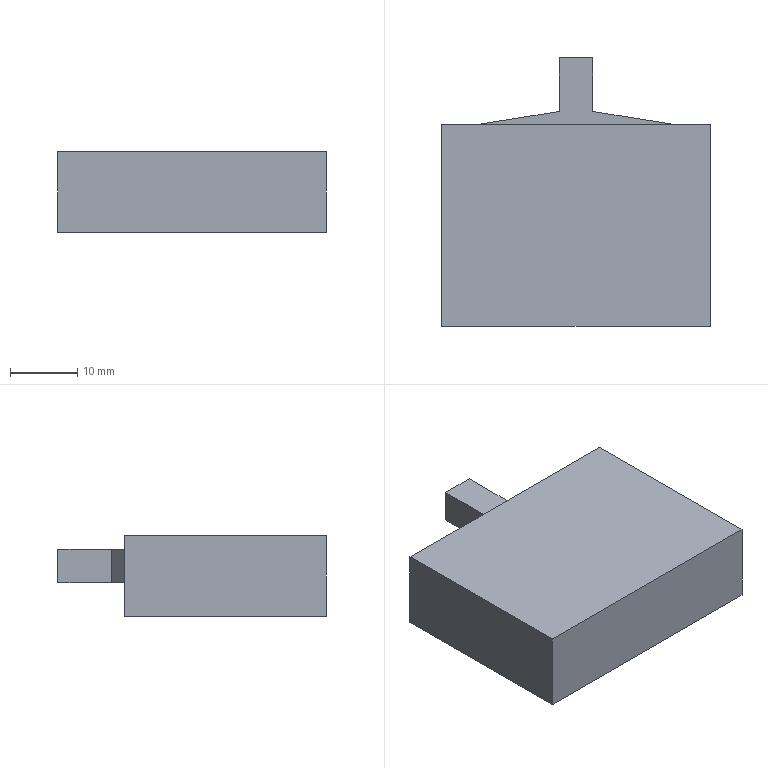Part | SolidWorks | features Extrusion 1, ICE 1 | 1 solid | 13 faces | box 40 x 40 x 12 mm | volume 14775 mm3 | plane 13
STEP:
#1=CARTESIAN_POINT('',(0.,0.,0.));
#2=VERTEX_POINT('',#1);
#3=CARTESIAN_POINT('',(0.,-30.,0.));
#4=VERTEX_POINT('',#3);
#5=CARTESIAN_POINT('',(0.,0.,0.));
#6=DIRECTION('',(0.,-1.,0.));
#7=VECTOR('',#6,1000.);
#8=LINE('',#5,#7);
#9=EDGE_CURVE('',#2,#4,#8,.T.);
#10=ORIENTED_EDGE('',*,*,#9,.T.);
#11=CARTESIAN_POINT('',(0.,-30.,12.));
#12=VERTEX_POINT('',#11);
#13=CARTESIAN_POINT('',(0.,-30.,12.));
#14=DIRECTION('',(0.,0.,-1.));
#15=VECTOR('',#14,1000.);
#16=LINE('',#13,#15);
#17=EDGE_CURVE('',#12,#4,#16,.T.);
#18=ORIENTED_EDGE('',*,*,#17,.F.);
#19=CARTESIAN_POINT('',(0.,0.,12.));
#20=VERTEX_POINT('',#19);
#21=CARTESIAN_POINT('',(0.,0.,12.));
#22=DIRECTION('',(0.,-1.,0.));
#23=VECTOR('',#22,1000.);
#24=LINE('',#21,#23);
#25=EDGE_CURVE('',#20,#12,#24,.T.);
#26=ORIENTED_EDGE('',*,*,#25,.F.);
#27=CARTESIAN_POINT('',(0.,0.,12.));
#28=DIRECTION('',(0.,0.,-1.));
#29=VECTOR('',#28,1000.);
#30=LINE('',#27,#29);
#31=EDGE_CURVE('',#20,#2,#30,.T.);
#32=ORIENTED_EDGE('',*,*,#31,.T.);
#33=EDGE_LOOP('',(#10,#18,#26,#32));
#34=FACE_OUTER_BOUND('',#33,.T.);
#35=CARTESIAN_POINT('',(0.,0.,12.));
#36=DIRECTION('',(1.,0.,0.));
#37=DIRECTION('',(0.,1.,0.));
#38=AXIS2_PLACEMENT_3D('',#35,#36,#37);
#39=PLANE('',#38);
#40=ADVANCED_FACE('',(#34),#39,.F.);
#41=CARTESIAN_POINT('',(40.,-30.,0.));
#42=VERTEX_POINT('',#41);
#43=CARTESIAN_POINT('',(0.,-30.,0.));
#44=DIRECTION('',(1.,0.,0.));
#45=VECTOR('',#44,1000.);
#46=LINE('',#43,#45);
#47=EDGE_CURVE('',#4,#42,#46,.T.);
#48=ORIENTED_EDGE('',*,*,#47,.T.);
#49=CARTESIAN_POINT('',(40.,-30.,12.));
#50=VERTEX_POINT('',#49);
#51=CARTESIAN_POINT('',(40.,-30.,12.));
#52=DIRECTION('',(0.,0.,-1.));
#53=VECTOR('',#52,1000.);
#54=LINE('',#51,#53);
#55=EDGE_CURVE('',#50,#42,#54,.T.);
#56=ORIENTED_EDGE('',*,*,#55,.F.);
#57=CARTESIAN_POINT('',(0.,-30.,12.));
#58=DIRECTION('',(1.,0.,0.));
#59=VECTOR('',#58,1000.);
#60=LINE('',#57,#59);
#61=EDGE_CURVE('',#12,#50,#60,.T.);
#62=ORIENTED_EDGE('',*,*,#61,.F.);
#63=ORIENTED_EDGE('',*,*,#17,.T.);
#64=EDGE_LOOP('',(#48,#56,#62,#63));
#65=FACE_OUTER_BOUND('',#64,.T.);
#66=CARTESIAN_POINT('',(0.,-30.,12.));
#67=DIRECTION('',(0.,1.,0.));
#68=DIRECTION('',(0.,0.,1.));
#69=AXIS2_PLACEMENT_3D('',#66,#67,#68);
#70=PLANE('',#69);
#71=ADVANCED_FACE('',(#65),#70,.F.);
#72=CARTESIAN_POINT('',(40.,0.,0.));
#73=VERTEX_POINT('',#72);
#74=CARTESIAN_POINT('',(40.,0.,0.));
#75=DIRECTION('',(0.,1.,0.));
#76=VECTOR('',#75,1000.);
#77=LINE('',#74,#76);
#78=EDGE_CURVE('',#42,#73,#77,.T.);
#79=ORIENTED_EDGE('',*,*,#78,.T.);
#80=CARTESIAN_POINT('',(40.,0.,12.));
#81=VERTEX_POINT('',#80);
#82=CARTESIAN_POINT('',(40.,0.,12.));
#83=DIRECTION('',(0.,0.,-1.));
#84=VECTOR('',#83,1000.);
#85=LINE('',#82,#84);
#86=EDGE_CURVE('',#81,#73,#85,.T.);
#87=ORIENTED_EDGE('',*,*,#86,.F.);
#88=CARTESIAN_POINT('',(40.,0.,12.));
#89=DIRECTION('',(0.,1.,0.));
#90=VECTOR('',#89,1000.);
#91=LINE('',#88,#90);
#92=EDGE_CURVE('',#50,#81,#91,.T.);
#93=ORIENTED_EDGE('',*,*,#92,.F.);
#94=ORIENTED_EDGE('',*,*,#55,.T.);
#95=EDGE_LOOP('',(#79,#87,#93,#94));
#96=FACE_OUTER_BOUND('',#95,.T.);
#97=CARTESIAN_POINT('',(40.,0.,12.));
#98=DIRECTION('',(-1.,0.,0.));
#99=DIRECTION('',(0.,-1.,0.));
#100=AXIS2_PLACEMENT_3D('',#97,#98,#99);
#101=PLANE('',#100);
#102=ADVANCED_FACE('',(#96),#101,.F.);
#103=CARTESIAN_POINT('',(5.,0.,10.));
#104=VERTEX_POINT('',#103);
#105=CARTESIAN_POINT('',(5.,0.,5.));
#106=VERTEX_POINT('',#105);
#107=CARTESIAN_POINT('',(5.,0.,10.));
#108=DIRECTION('',(0.,0.,-1.));
#109=VECTOR('',#108,1000.);
#110=LINE('',#107,#109);
#111=EDGE_CURVE('',#104,#106,#110,.T.);
#112=ORIENTED_EDGE('',*,*,#111,.T.);
#113=CARTESIAN_POINT('',(35.,0.,5.));
#114=VERTEX_POINT('',#113);
#115=CARTESIAN_POINT('',(0.,0.,5.));
#116=DIRECTION('',(1.,0.,0.));
#117=VECTOR('',#116,1000.);
#118=LINE('',#115,#117);
#119=EDGE_CURVE('',#106,#114,#118,.T.);
#120=ORIENTED_EDGE('',*,*,#119,.T.);
#121=CARTESIAN_POINT('',(35.,0.,10.));
#122=VERTEX_POINT('',#121);
#123=CARTESIAN_POINT('',(35.,0.,10.));
#124=DIRECTION('',(0.,0.,-1.));
#125=VECTOR('',#124,1000.);
#126=LINE('',#123,#125);
#127=EDGE_CURVE('',#122,#114,#126,.T.);
#128=ORIENTED_EDGE('',*,*,#127,.F.);
#129=CARTESIAN_POINT('',(0.,0.,10.));
#130=DIRECTION('',(1.,0.,0.));
#131=VECTOR('',#130,1000.);
#132=LINE('',#129,#131);
#133=EDGE_CURVE('',#104,#122,#132,.T.);
#134=ORIENTED_EDGE('',*,*,#133,.F.);
#135=EDGE_LOOP('',(#112,#120,#128,#134));
#136=FACE_BOUND('',#135,.T.);
#137=CARTESIAN_POINT('',(0.,0.,0.));
#138=DIRECTION('',(-1.,0.,0.));
#139=VECTOR('',#138,1000.);
#140=LINE('',#137,#139);
#141=EDGE_CURVE('',#73,#2,#140,.T.);
#142=ORIENTED_EDGE('',*,*,#141,.T.);
#143=ORIENTED_EDGE('',*,*,#31,.F.);
#144=CARTESIAN_POINT('',(0.,0.,12.));
#145=DIRECTION('',(-1.,0.,0.));
#146=VECTOR('',#145,1000.);
#147=LINE('',#144,#146);
#148=EDGE_CURVE('',#81,#20,#147,.T.);
#149=ORIENTED_EDGE('',*,*,#148,.F.);
#150=ORIENTED_EDGE('',*,*,#86,.T.);
#151=EDGE_LOOP('',(#142,#143,#149,#150));
#152=FACE_OUTER_BOUND('',#151,.T.);
#153=CARTESIAN_POINT('',(0.,0.,12.));
#154=DIRECTION('',(0.,-1.,0.));
#155=DIRECTION('',(0.,0.,-1.));
#156=AXIS2_PLACEMENT_3D('',#153,#154,#155);
#157=PLANE('',#156);
#158=ADVANCED_FACE('',(#136,#152),#157,.F.);
#159=ORIENTED_EDGE('',*,*,#25,.T.);
#160=ORIENTED_EDGE('',*,*,#61,.T.);
#161=ORIENTED_EDGE('',*,*,#92,.T.);
#162=ORIENTED_EDGE('',*,*,#148,.T.);
#163=EDGE_LOOP('',(#159,#160,#161,#162));
#164=FACE_OUTER_BOUND('',#163,.T.);
#165=CARTESIAN_POINT('',(0.,0.,12.));
#166=DIRECTION('',(0.,0.,1.));
#167=DIRECTION('',(1.,0.,0.));
#168=AXIS2_PLACEMENT_3D('',#165,#166,#167);
#169=PLANE('',#168);
#170=ADVANCED_FACE('',(#164),#169,.T.);
#171=ORIENTED_EDGE('',*,*,#9,.F.);
#172=ORIENTED_EDGE('',*,*,#141,.F.);
#173=ORIENTED_EDGE('',*,*,#78,.F.);
#174=ORIENTED_EDGE('',*,*,#47,.F.);
#175=EDGE_LOOP('',(#171,#172,#173,#174));
#176=FACE_OUTER_BOUND('',#175,.T.);
#177=CARTESIAN_POINT('',(0.,0.,0.));
#178=DIRECTION('',(0.,0.,1.));
#179=DIRECTION('',(1.,0.,0.));
#180=AXIS2_PLACEMENT_3D('',#177,#178,#179);
#181=PLANE('',#180);
#182=ADVANCED_FACE('',(#176),#181,.F.);
#183=CARTESIAN_POINT('',(17.5,2.,5.));
#184=VERTEX_POINT('',#183);
#185=CARTESIAN_POINT('',(0.1248,-0.78,5.));
#186=DIRECTION('',(-0.9874,-0.158,0.));
#187=VECTOR('',#186,1000.);
#188=LINE('',#185,#187);
#189=EDGE_CURVE('',#184,#106,#188,.T.);
#190=ORIENTED_EDGE('',*,*,#189,.T.);
#191=ORIENTED_EDGE('',*,*,#111,.F.);
#192=CARTESIAN_POINT('',(17.5,2.,10.));
#193=VERTEX_POINT('',#192);
#194=CARTESIAN_POINT('',(0.1248,-0.78,10.));
#195=DIRECTION('',(-0.9874,-0.158,0.));
#196=VECTOR('',#195,1000.);
#197=LINE('',#194,#196);
#198=EDGE_CURVE('',#193,#104,#197,.T.);
#199=ORIENTED_EDGE('',*,*,#198,.F.);
#200=CARTESIAN_POINT('',(17.5,2.,10.));
#201=DIRECTION('',(0.,0.,-1.));
#202=VECTOR('',#201,1000.);
#203=LINE('',#200,#202);
#204=EDGE_CURVE('',#193,#184,#203,.T.);
#205=ORIENTED_EDGE('',*,*,#204,.T.);
#206=EDGE_LOOP('',(#190,#191,#199,#205));
#207=FACE_OUTER_BOUND('',#206,.T.);
#208=CARTESIAN_POINT('',(0.1248,-0.78,10.));
#209=DIRECTION('',(0.158,-0.9874,0.));
#210=DIRECTION('',(0.9874,0.158,0.));
#211=AXIS2_PLACEMENT_3D('',#208,#209,#210);
#212=PLANE('',#211);
#213=ADVANCED_FACE('',(#207),#212,.F.);
#214=CARTESIAN_POINT('',(22.5,2.,5.));
#215=VERTEX_POINT('',#214);
#216=CARTESIAN_POINT('',(0.8736,5.46,5.));
#217=DIRECTION('',(0.9874,-0.158,0.));
#218=VECTOR('',#217,1000.);
#219=LINE('',#216,#218);
#220=EDGE_CURVE('',#215,#114,#219,.T.);
#221=ORIENTED_EDGE('',*,*,#220,.F.);
#222=CARTESIAN_POINT('',(22.5,2.,10.));
#223=VERTEX_POINT('',#222);
#224=CARTESIAN_POINT('',(22.5,2.,10.));
#225=DIRECTION('',(0.,0.,-1.));
#226=VECTOR('',#225,1000.);
#227=LINE('',#224,#226);
#228=EDGE_CURVE('',#223,#215,#227,.T.);
#229=ORIENTED_EDGE('',*,*,#228,.F.);
#230=CARTESIAN_POINT('',(0.8736,5.46,10.));
#231=DIRECTION('',(0.9874,-0.158,0.));
#232=VECTOR('',#231,1000.);
#233=LINE('',#230,#232);
#234=EDGE_CURVE('',#223,#122,#233,.T.);
#235=ORIENTED_EDGE('',*,*,#234,.T.);
#236=ORIENTED_EDGE('',*,*,#127,.T.);
#237=EDGE_LOOP('',(#221,#229,#235,#236));
#238=FACE_OUTER_BOUND('',#237,.T.);
#239=CARTESIAN_POINT('',(0.8736,5.46,10.));
#240=DIRECTION('',(0.158,0.9874,0.));
#241=DIRECTION('',(-0.9874,0.158,0.));
#242=AXIS2_PLACEMENT_3D('',#239,#240,#241);
#243=PLANE('',#242);
#244=ADVANCED_FACE('',(#238),#243,.T.);
#245=CARTESIAN_POINT('',(22.5,10.,5.));
#246=VERTEX_POINT('',#245);
#247=CARTESIAN_POINT('',(22.5,0.,5.));
#248=DIRECTION('',(0.,1.,0.));
#249=VECTOR('',#248,1000.);
#250=LINE('',#247,#249);
#251=EDGE_CURVE('',#215,#246,#250,.T.);
#252=ORIENTED_EDGE('',*,*,#251,.T.);
#253=CARTESIAN_POINT('',(22.5,10.,10.));
#254=VERTEX_POINT('',#253);
#255=CARTESIAN_POINT('',(22.5,10.,10.));
#256=DIRECTION('',(0.,0.,-1.));
#257=VECTOR('',#256,1000.);
#258=LINE('',#255,#257);
#259=EDGE_CURVE('',#254,#246,#258,.T.);
#260=ORIENTED_EDGE('',*,*,#259,.F.);
#261=CARTESIAN_POINT('',(22.5,0.,10.));
#262=DIRECTION('',(0.,1.,0.));
#263=VECTOR('',#262,1000.);
#264=LINE('',#261,#263);
#265=EDGE_CURVE('',#223,#254,#264,.T.);
#266=ORIENTED_EDGE('',*,*,#265,.F.);
#267=ORIENTED_EDGE('',*,*,#228,.T.);
#268=EDGE_LOOP('',(#252,#260,#266,#267));
#269=FACE_OUTER_BOUND('',#268,.T.);
#270=CARTESIAN_POINT('',(22.5,0.,10.));
#271=DIRECTION('',(-1.,0.,0.));
#272=DIRECTION('',(0.,-1.,0.));
#273=AXIS2_PLACEMENT_3D('',#270,#271,#272);
#274=PLANE('',#273);
#275=ADVANCED_FACE('',(#269),#274,.F.);
#276=CARTESIAN_POINT('',(17.5,10.,5.));
#277=VERTEX_POINT('',#276);
#278=CARTESIAN_POINT('',(0.,10.,5.));
#279=DIRECTION('',(-1.,0.,0.));
#280=VECTOR('',#279,1000.);
#281=LINE('',#278,#280);
#282=EDGE_CURVE('',#246,#277,#281,.T.);
#283=ORIENTED_EDGE('',*,*,#282,.T.);
#284=CARTESIAN_POINT('',(17.5,10.,10.));
#285=VERTEX_POINT('',#284);
#286=CARTESIAN_POINT('',(17.5,10.,10.));
#287=DIRECTION('',(0.,0.,-1.));
#288=VECTOR('',#287,1000.);
#289=LINE('',#286,#288);
#290=EDGE_CURVE('',#285,#277,#289,.T.);
#291=ORIENTED_EDGE('',*,*,#290,.F.);
#292=CARTESIAN_POINT('',(0.,10.,10.));
#293=DIRECTION('',(-1.,0.,0.));
#294=VECTOR('',#293,1000.);
#295=LINE('',#292,#294);
#296=EDGE_CURVE('',#254,#285,#295,.T.);
#297=ORIENTED_EDGE('',*,*,#296,.F.);
#298=ORIENTED_EDGE('',*,*,#259,.T.);
#299=EDGE_LOOP('',(#283,#291,#297,#298));
#300=FACE_OUTER_BOUND('',#299,.T.);
#301=CARTESIAN_POINT('',(0.,10.,10.));
#302=DIRECTION('',(0.,-1.,0.));
#303=DIRECTION('',(0.,0.,-1.));
#304=AXIS2_PLACEMENT_3D('',#301,#302,#303);
#305=PLANE('',#304);
#306=ADVANCED_FACE('',(#300),#305,.F.);
#307=CARTESIAN_POINT('',(17.5,0.,5.));
#308=DIRECTION('',(0.,-1.,0.));
#309=VECTOR('',#308,1000.);
#310=LINE('',#307,#309);
#311=EDGE_CURVE('',#277,#184,#310,.T.);
#312=ORIENTED_EDGE('',*,*,#311,.T.);
#313=ORIENTED_EDGE('',*,*,#204,.F.);
#314=CARTESIAN_POINT('',(17.5,0.,10.));
#315=DIRECTION('',(0.,-1.,0.));
#316=VECTOR('',#315,1000.);
#317=LINE('',#314,#316);
#318=EDGE_CURVE('',#285,#193,#317,.T.);
#319=ORIENTED_EDGE('',*,*,#318,.F.);
#320=ORIENTED_EDGE('',*,*,#290,.T.);
#321=EDGE_LOOP('',(#312,#313,#319,#320));
#322=FACE_OUTER_BOUND('',#321,.T.);
#323=CARTESIAN_POINT('',(17.5,0.,10.));
#324=DIRECTION('',(1.,0.,0.));
#325=DIRECTION('',(0.,1.,0.));
#326=AXIS2_PLACEMENT_3D('',#323,#324,#325);
#327=PLANE('',#326);
#328=ADVANCED_FACE('',(#322),#327,.F.);
#329=ORIENTED_EDGE('',*,*,#198,.T.);
#330=ORIENTED_EDGE('',*,*,#133,.T.);
#331=ORIENTED_EDGE('',*,*,#234,.F.);
#332=ORIENTED_EDGE('',*,*,#265,.T.);
#333=ORIENTED_EDGE('',*,*,#296,.T.);
#334=ORIENTED_EDGE('',*,*,#318,.T.);
#335=EDGE_LOOP('',(#329,#330,#331,#332,#333,#334));
#336=FACE_OUTER_BOUND('',#335,.T.);
#337=CARTESIAN_POINT('',(0.,0.,10.));
#338=DIRECTION('',(0.,0.,-1.));
#339=DIRECTION('',(-1.,0.,0.));
#340=AXIS2_PLACEMENT_3D('',#337,#338,#339);
#341=PLANE('',#340);
#342=ADVANCED_FACE('',(#336),#341,.F.);
#343=ORIENTED_EDGE('',*,*,#189,.F.);
#344=ORIENTED_EDGE('',*,*,#311,.F.);
#345=ORIENTED_EDGE('',*,*,#282,.F.);
#346=ORIENTED_EDGE('',*,*,#251,.F.);
#347=ORIENTED_EDGE('',*,*,#220,.T.);
#348=ORIENTED_EDGE('',*,*,#119,.F.);
#349=EDGE_LOOP('',(#343,#344,#345,#346,#347,#348));
#350=FACE_OUTER_BOUND('',#349,.T.);
#351=CARTESIAN_POINT('',(0.,0.,5.));
#352=DIRECTION('',(0.,0.,-1.));
#353=DIRECTION('',(-1.,0.,0.));
#354=AXIS2_PLACEMENT_3D('',#351,#352,#353);
#355=PLANE('',#354);
#356=ADVANCED_FACE('',(#350),#355,.T.);
#357=CLOSED_SHELL('',(#40,#71,#102,#158,#170,#182,#213,#244,#275,#306,#328,#342,#356));
#358=MANIFOLD_SOLID_BREP('',#357);
#359=CARTESIAN_POINT('',(0.,0.,0.));
#360=DIRECTION('',(0.,0.,1.));
#361=DIRECTION('',(1.,0.,0.));
#362=AXIS2_PLACEMENT_3D('',#359,#360,#361);
#363=(LENGTH_UNIT()NAMED_UNIT(*)SI_UNIT(.MILLI.,.METRE.));
#364=UNCERTAINTY_MEASURE_WITH_UNIT(LENGTH_MEASURE(0.00001),#363,'','');
#365=(NAMED_UNIT(*)PLANE_ANGLE_UNIT()SI_UNIT($,.RADIAN.));
#366=(NAMED_UNIT(*)SI_UNIT($,.STERADIAN.)SOLID_ANGLE_UNIT());
#367=(GEOMETRIC_REPRESENTATION_CONTEXT(3)GLOBAL_UNCERTAINTY_ASSIGNED_CONTEXT((#364))GLOBAL_UNIT_ASSIGNED_CONTEXT((#363,#365,#366))REPRESENTATION_CONTEXT('',''));
#368=ADVANCED_BREP_SHAPE_REPRESENTATION('',(#358,#362),#367);